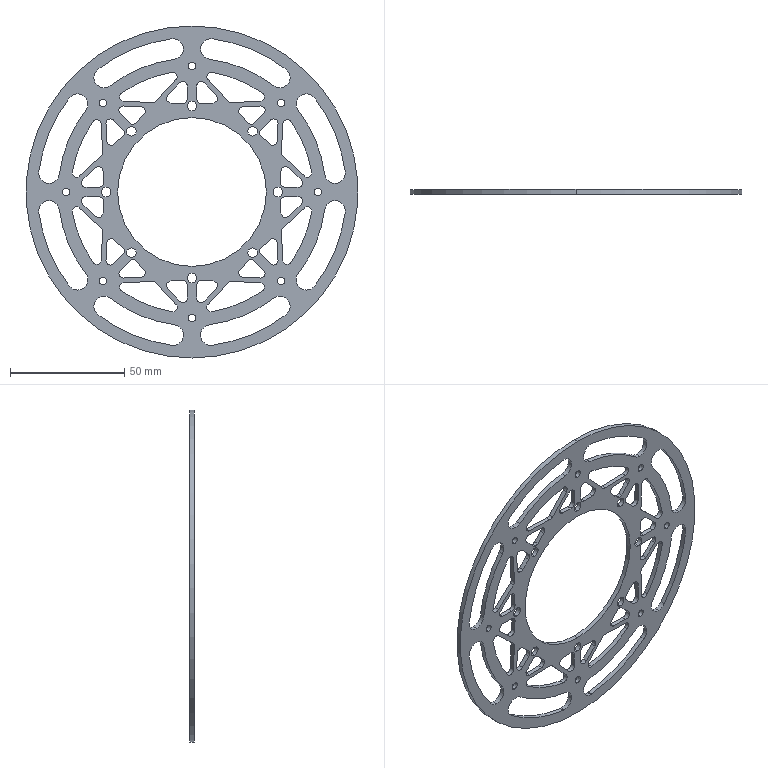Part | SolidWorks | features CirPattern 1, Extrusion 1, Fillet 1, ICE 1 | 1 solid | 244 faces | box 145 x 2 x 145 mm | volume 15235 mm3 | cylinder 178 | plane 66 | commonest cylinder face diameters 4 x94 9 x24 3.2 x16 4.2 x16 106 x8 117 x8